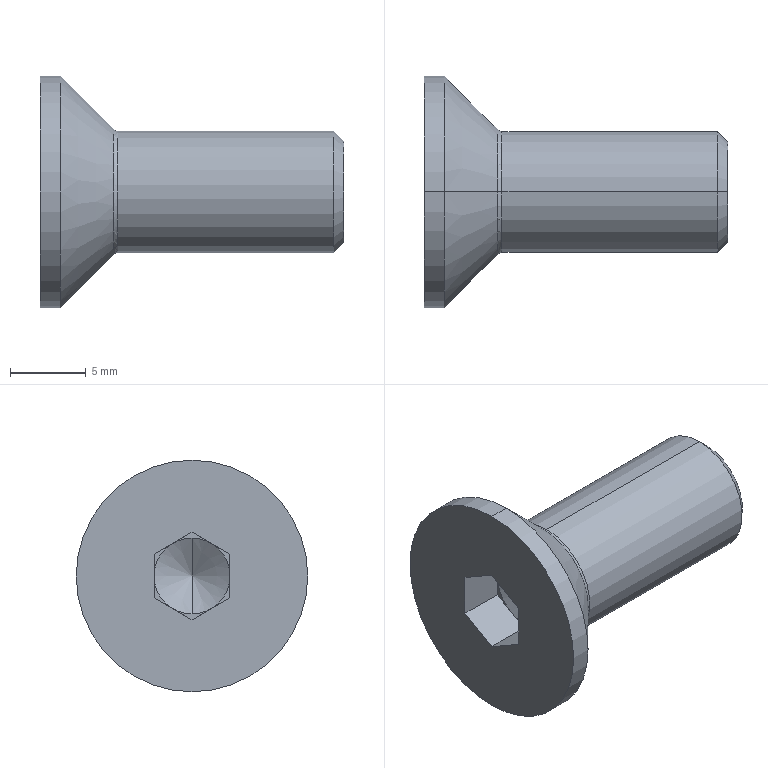Part | SolidWorks | features RevCut 3, Chamfer 1, Cut 1, Fillet 1, LPattern 1, Revolution 1 | 1 solid | 26 faces | box 20 x 15.24 x 15.24 mm | volume 1317 mm3 | plane 14 | cone 6 | cylinder 4 | torus 2 | commonest cylinder face diameters 8 x2 15.24 x2
STEP:
#1=CARTESIAN_POINT('',(4.443,0.,0.));
#2=VERTEX_POINT('',#1);
#3=CARTESIAN_POINT('',(3.,0.,2.5));
#4=VERTEX_POINT('',#3);
#5=CARTESIAN_POINT('',(4.443,0.,0.));
#6=DIRECTION('',(-0.5,0.,0.866));
#7=VECTOR('',#6,1000.);
#8=LINE('',#5,#7);
#9=EDGE_CURVE('',#2,#4,#8,.T.);
#10=ORIENTED_EDGE('',*,*,#9,.F.);
#11=CARTESIAN_POINT('',(3.,0.,-2.5));
#12=VERTEX_POINT('',#11);
#13=CARTESIAN_POINT('',(4.443,0.,0.));
#14=DIRECTION('',(-0.5,0.,-0.866));
#15=VECTOR('',#14,1000.);
#16=LINE('',#13,#15);
#17=EDGE_CURVE('',#2,#12,#16,.T.);
#18=ORIENTED_EDGE('',*,*,#17,.T.);
#19=CARTESIAN_POINT('',(3.,-1.25,-2.165));
#20=VERTEX_POINT('',#19);
#21=CARTESIAN_POINT('',(3.,0.,0.));
#22=DIRECTION('',(-1.,0.,0.));
#23=DIRECTION('',(0.,0.,1.));
#24=AXIS2_PLACEMENT_3D('',#21,#22,#23);
#25=CIRCLE('',#24,2.5);
#26=EDGE_CURVE('',#12,#20,#25,.T.);
#27=ORIENTED_EDGE('',*,*,#26,.T.);
#28=CARTESIAN_POINT('',(3.,-2.5,0.));
#29=VERTEX_POINT('',#28);
#30=CARTESIAN_POINT('',(3.,0.,0.));
#31=DIRECTION('',(-1.,0.,0.));
#32=DIRECTION('',(0.,0.,1.));
#33=AXIS2_PLACEMENT_3D('',#30,#31,#32);
#34=CIRCLE('',#33,2.5);
#35=EDGE_CURVE('',#20,#29,#34,.T.);
#36=ORIENTED_EDGE('',*,*,#35,.T.);
#37=CARTESIAN_POINT('',(3.,-1.25,2.165));
#38=VERTEX_POINT('',#37);
#39=CARTESIAN_POINT('',(3.,0.,0.));
#40=DIRECTION('',(-1.,0.,0.));
#41=DIRECTION('',(0.,0.,1.));
#42=AXIS2_PLACEMENT_3D('',#39,#40,#41);
#43=CIRCLE('',#42,2.5);
#44=EDGE_CURVE('',#29,#38,#43,.T.);
#45=ORIENTED_EDGE('',*,*,#44,.T.);
#46=CARTESIAN_POINT('',(3.,0.,0.));
#47=DIRECTION('',(-1.,0.,0.));
#48=DIRECTION('',(0.,0.,1.));
#49=AXIS2_PLACEMENT_3D('',#46,#47,#48);
#50=CIRCLE('',#49,2.5);
#51=EDGE_CURVE('',#38,#4,#50,.T.);
#52=ORIENTED_EDGE('',*,*,#51,.T.);
#53=EDGE_LOOP('',(#10,#18,#27,#36,#45,#52));
#54=FACE_OUTER_BOUND('',#53,.T.);
#55=CARTESIAN_POINT('',(-995.557,0.,0.));
#56=DIRECTION('',(-1.,0.,0.));
#57=DIRECTION('',(0.,0.,1.));
#58=AXIS2_PLACEMENT_3D('',#55,#56,#57);
#59=CONICAL_SURFACE('',#58,1732.051,1.047);
#60=ADVANCED_FACE('',(#54),#59,.F.);
#61=CARTESIAN_POINT('',(0.,0.,7.62));
#62=VERTEX_POINT('',#61);
#63=CARTESIAN_POINT('',(0.,0.,-7.62));
#64=VERTEX_POINT('',#63);
#65=CARTESIAN_POINT('',(0.,0.,0.));
#66=DIRECTION('',(-1.,0.,0.));
#67=DIRECTION('',(0.,0.,-1.));
#68=AXIS2_PLACEMENT_3D('',#65,#66,#67);
#69=CIRCLE('',#68,7.62);
#70=EDGE_CURVE('',#62,#64,#69,.T.);
#71=ORIENTED_EDGE('',*,*,#70,.F.);
#72=CARTESIAN_POINT('',(1.34,0.,7.62));
#73=VERTEX_POINT('',#72);
#74=CARTESIAN_POINT('',(11.853,0.,7.62));
#75=DIRECTION('',(1.,0.,0.));
#76=VECTOR('',#75,1000.);
#77=LINE('',#74,#76);
#78=EDGE_CURVE('',#62,#73,#77,.T.);
#79=ORIENTED_EDGE('',*,*,#78,.T.);
#80=CARTESIAN_POINT('',(1.34,0.,-7.62));
#81=VERTEX_POINT('',#80);
#82=CARTESIAN_POINT('',(1.34,0.,0.));
#83=DIRECTION('',(1.,0.,0.));
#84=DIRECTION('',(0.,0.,1.));
#85=AXIS2_PLACEMENT_3D('',#82,#83,#84);
#86=CIRCLE('',#85,7.62);
#87=EDGE_CURVE('',#81,#73,#86,.T.);
#88=ORIENTED_EDGE('',*,*,#87,.F.);
#89=CARTESIAN_POINT('',(11.853,0.,-7.62));
#90=DIRECTION('',(1.,0.,0.));
#91=VECTOR('',#90,1000.);
#92=LINE('',#89,#91);
#93=EDGE_CURVE('',#64,#81,#92,.T.);
#94=ORIENTED_EDGE('',*,*,#93,.F.);
#95=EDGE_LOOP('',(#71,#79,#88,#94));
#96=FACE_OUTER_BOUND('',#95,.T.);
#97=CARTESIAN_POINT('',(11.853,0.,0.));
#98=DIRECTION('',(1.,0.,0.));
#99=DIRECTION('',(0.,0.,-1.));
#100=AXIS2_PLACEMENT_3D('',#97,#98,#99);
#101=CYLINDRICAL_SURFACE('',#100,7.62);
#102=ADVANCED_FACE('',(#96),#101,.T.);
#103=CARTESIAN_POINT('',(20.,0.,-3.323));
#104=VERTEX_POINT('',#103);
#105=CARTESIAN_POINT('',(20.,0.,3.323));
#106=VERTEX_POINT('',#105);
#107=CARTESIAN_POINT('',(20.,0.,0.));
#108=DIRECTION('',(1.,0.,0.));
#109=DIRECTION('',(0.,0.,1.));
#110=AXIS2_PLACEMENT_3D('',#107,#108,#109);
#111=CIRCLE('',#110,3.323);
#112=EDGE_CURVE('',#104,#106,#111,.T.);
#113=ORIENTED_EDGE('',*,*,#112,.F.);
#114=CARTESIAN_POINT('',(19.323,0.,-4.));
#115=VERTEX_POINT('',#114);
#116=CARTESIAN_POINT('',(19.323,0.,-4.));
#117=DIRECTION('',(-0.7071,0.,-0.7071));
#118=VECTOR('',#117,1000.);
#119=LINE('',#116,#118);
#120=EDGE_CURVE('',#104,#115,#119,.T.);
#121=ORIENTED_EDGE('',*,*,#120,.T.);
#122=CARTESIAN_POINT('',(19.323,0.,4.));
#123=VERTEX_POINT('',#122);
#124=CARTESIAN_POINT('',(19.323,0.,0.));
#125=DIRECTION('',(-1.,0.,0.));
#126=DIRECTION('',(0.,0.,1.));
#127=AXIS2_PLACEMENT_3D('',#124,#125,#126);
#128=CIRCLE('',#127,4.);
#129=EDGE_CURVE('',#123,#115,#128,.T.);
#130=ORIENTED_EDGE('',*,*,#129,.F.);
#131=CARTESIAN_POINT('',(19.323,0.,4.));
#132=DIRECTION('',(-0.7071,0.,0.7071));
#133=VECTOR('',#132,1000.);
#134=LINE('',#131,#133);
#135=EDGE_CURVE('',#106,#123,#134,.T.);
#136=ORIENTED_EDGE('',*,*,#135,.F.);
#137=EDGE_LOOP('',(#113,#121,#130,#136));
#138=FACE_OUTER_BOUND('',#137,.T.);
#139=CARTESIAN_POINT('',(19.323,0.,0.));
#140=DIRECTION('',(-1.,0.,0.));
#141=DIRECTION('',(0.,0.,1.));
#142=AXIS2_PLACEMENT_3D('',#139,#140,#141);
#143=CONICAL_SURFACE('',#142,4.,0.7854);
#144=ADVANCED_FACE('',(#138),#143,.T.);
#145=CARTESIAN_POINT('',(4.843,0.,-4.117));
#146=VERTEX_POINT('',#145);
#147=CARTESIAN_POINT('',(4.843,0.,4.117));
#148=VERTEX_POINT('',#147);
#149=CARTESIAN_POINT('',(4.843,0.,0.));
#150=DIRECTION('',(-1.,0.,0.));
#151=DIRECTION('',(0.,0.,1.));
#152=AXIS2_PLACEMENT_3D('',#149,#150,#151);
#153=CIRCLE('',#152,4.117);
#154=EDGE_CURVE('',#146,#148,#153,.T.);
#155=ORIENTED_EDGE('',*,*,#154,.F.);
#156=CARTESIAN_POINT('',(5.126,0.,-4.));
#157=VERTEX_POINT('',#156);
#158=CARTESIAN_POINT('',(5.126,0.,-4.4));
#159=DIRECTION('',(0.,1.,0.));
#160=DIRECTION('',(0.,0.,1.));
#161=AXIS2_PLACEMENT_3D('',#158,#159,#160);
#162=CIRCLE('',#161,0.4);
#163=EDGE_CURVE('',#146,#157,#162,.T.);
#164=ORIENTED_EDGE('',*,*,#163,.T.);
#165=CARTESIAN_POINT('',(5.126,0.,4.));
#166=VERTEX_POINT('',#165);
#167=CARTESIAN_POINT('',(5.126,0.,0.));
#168=DIRECTION('',(1.,0.,0.));
#169=DIRECTION('',(0.,0.,1.));
#170=AXIS2_PLACEMENT_3D('',#167,#168,#169);
#171=CIRCLE('',#170,4.);
#172=EDGE_CURVE('',#166,#157,#171,.T.);
#173=ORIENTED_EDGE('',*,*,#172,.F.);
#174=CARTESIAN_POINT('',(5.126,0.,4.4));
#175=DIRECTION('',(0.,-1.,0.));
#176=DIRECTION('',(0.,0.,-1.));
#177=AXIS2_PLACEMENT_3D('',#174,#175,#176);
#178=CIRCLE('',#177,0.4);
#179=EDGE_CURVE('',#148,#166,#178,.T.);
#180=ORIENTED_EDGE('',*,*,#179,.F.);
#181=EDGE_LOOP('',(#155,#164,#173,#180));
#182=FACE_OUTER_BOUND('',#181,.T.);
#183=CARTESIAN_POINT('',(5.126,0.,0.));
#184=DIRECTION('',(-1.,0.,0.));
#185=DIRECTION('',(0.,0.,1.));
#186=AXIS2_PLACEMENT_3D('',#183,#184,#185);
#187=TOROIDAL_SURFACE('',#186,4.4,0.4);
#188=ADVANCED_FACE('',(#182),#187,.F.);
#189=ORIENTED_EDGE('',*,*,#129,.T.);
#190=CARTESIAN_POINT('',(-0.5871,0.,-4.));
#191=DIRECTION('',(-1.,0.,0.));
#192=VECTOR('',#191,1000.);
#193=LINE('',#190,#192);
#194=EDGE_CURVE('',#115,#157,#193,.T.);
#195=ORIENTED_EDGE('',*,*,#194,.T.);
#196=CARTESIAN_POINT('',(5.126,0.,0.));
#197=DIRECTION('',(1.,0.,0.));
#198=DIRECTION('',(0.,0.,1.));
#199=AXIS2_PLACEMENT_3D('',#196,#197,#198);
#200=CIRCLE('',#199,4.);
#201=EDGE_CURVE('',#157,#166,#200,.T.);
#202=ORIENTED_EDGE('',*,*,#201,.T.);
#203=CARTESIAN_POINT('',(-0.5871,0.,4.));
#204=DIRECTION('',(-1.,0.,0.));
#205=VECTOR('',#204,1000.);
#206=LINE('',#203,#205);
#207=EDGE_CURVE('',#123,#166,#206,.T.);
#208=ORIENTED_EDGE('',*,*,#207,.F.);
#209=EDGE_LOOP('',(#189,#195,#202,#208));
#210=FACE_OUTER_BOUND('',#209,.T.);
#211=CARTESIAN_POINT('',(-0.5871,0.,0.));
#212=DIRECTION('',(-1.,0.,0.));
#213=DIRECTION('',(0.,0.,1.));
#214=AXIS2_PLACEMENT_3D('',#211,#212,#213);
#215=CYLINDRICAL_SURFACE('',#214,4.);
#216=ADVANCED_FACE('',(#210),#215,.T.);
#217=CARTESIAN_POINT('',(4.843,0.,0.));
#218=DIRECTION('',(-1.,0.,0.));
#219=DIRECTION('',(0.,0.,1.));
#220=AXIS2_PLACEMENT_3D('',#217,#218,#219);
#221=CIRCLE('',#220,4.117);
#222=EDGE_CURVE('',#148,#146,#221,.T.);
#223=ORIENTED_EDGE('',*,*,#222,.T.);
#224=CARTESIAN_POINT('',(4.96,0.,-4.));
#225=DIRECTION('',(-0.7071,0.,-0.7071));
#226=VECTOR('',#225,1000.);
#227=LINE('',#224,#226);
#228=EDGE_CURVE('',#146,#81,#227,.T.);
#229=ORIENTED_EDGE('',*,*,#228,.T.);
#230=ORIENTED_EDGE('',*,*,#87,.T.);
#231=CARTESIAN_POINT('',(4.96,0.,4.));
#232=DIRECTION('',(-0.7071,0.,0.7071));
#233=VECTOR('',#232,1000.);
#234=LINE('',#231,#233);
#235=EDGE_CURVE('',#148,#73,#234,.T.);
#236=ORIENTED_EDGE('',*,*,#235,.F.);
#237=EDGE_LOOP('',(#223,#229,#230,#236));
#238=FACE_OUTER_BOUND('',#237,.T.);
#239=CARTESIAN_POINT('',(4.96,0.,0.));
#240=DIRECTION('',(-1.,0.,0.));
#241=DIRECTION('',(0.,0.,1.));
#242=AXIS2_PLACEMENT_3D('',#239,#240,#241);
#243=CONICAL_SURFACE('',#242,4.,0.7854);
#244=ADVANCED_FACE('',(#238),#243,.T.);
#245=ORIENTED_EDGE('',*,*,#228,.F.);
#246=ORIENTED_EDGE('',*,*,#154,.T.);
#247=ORIENTED_EDGE('',*,*,#235,.T.);
#248=CARTESIAN_POINT('',(1.34,0.,0.));
#249=DIRECTION('',(1.,0.,0.));
#250=DIRECTION('',(0.,0.,1.));
#251=AXIS2_PLACEMENT_3D('',#248,#249,#250);
#252=CIRCLE('',#251,7.62);
#253=EDGE_CURVE('',#73,#81,#252,.T.);
#254=ORIENTED_EDGE('',*,*,#253,.T.);
#255=EDGE_LOOP('',(#245,#246,#247,#254));
#256=FACE_OUTER_BOUND('',#255,.T.);
#257=CARTESIAN_POINT('',(4.96,0.,0.));
#258=DIRECTION('',(-1.,0.,0.));
#259=DIRECTION('',(0.,0.,1.));
#260=AXIS2_PLACEMENT_3D('',#257,#258,#259);
#261=CONICAL_SURFACE('',#260,4.,0.7854);
#262=ADVANCED_FACE('',(#256),#261,.T.);
#263=ORIENTED_EDGE('',*,*,#194,.F.);
#264=CARTESIAN_POINT('',(19.323,0.,0.));
#265=DIRECTION('',(-1.,0.,0.));
#266=DIRECTION('',(0.,0.,1.));
#267=AXIS2_PLACEMENT_3D('',#264,#265,#266);
#268=CIRCLE('',#267,4.);
#269=EDGE_CURVE('',#115,#123,#268,.T.);
#270=ORIENTED_EDGE('',*,*,#269,.T.);
#271=ORIENTED_EDGE('',*,*,#207,.T.);
#272=ORIENTED_EDGE('',*,*,#172,.T.);
#273=EDGE_LOOP('',(#263,#270,#271,#272));
#274=FACE_OUTER_BOUND('',#273,.T.);
#275=CARTESIAN_POINT('',(-0.5871,0.,0.));
#276=DIRECTION('',(-1.,0.,0.));
#277=DIRECTION('',(0.,0.,1.));
#278=AXIS2_PLACEMENT_3D('',#275,#276,#277);
#279=CYLINDRICAL_SURFACE('',#278,4.);
#280=ADVANCED_FACE('',(#274),#279,.T.);
#281=CARTESIAN_POINT('',(20.,0.,0.));
#282=DIRECTION('',(1.,0.,0.));
#283=DIRECTION('',(0.,0.,1.));
#284=AXIS2_PLACEMENT_3D('',#281,#282,#283);
#285=CIRCLE('',#284,3.323);
#286=EDGE_CURVE('',#106,#104,#285,.T.);
#287=ORIENTED_EDGE('',*,*,#286,.T.);
#288=ORIENTED_EDGE('',*,*,#112,.T.);
#289=EDGE_LOOP('',(#287,#288));
#290=FACE_OUTER_BOUND('',#289,.T.);
#291=CARTESIAN_POINT('',(20.,4.,0.));
#292=DIRECTION('',(-1.,0.,0.));
#293=DIRECTION('',(0.,0.,1.));
#294=AXIS2_PLACEMENT_3D('',#291,#292,#293);
#295=PLANE('',#294);
#296=ADVANCED_FACE('',(#290),#295,.F.);
#297=ORIENTED_EDGE('',*,*,#163,.F.);
#298=ORIENTED_EDGE('',*,*,#222,.F.);
#299=ORIENTED_EDGE('',*,*,#179,.T.);
#300=ORIENTED_EDGE('',*,*,#201,.F.);
#301=EDGE_LOOP('',(#297,#298,#299,#300));
#302=FACE_OUTER_BOUND('',#301,.T.);
#303=CARTESIAN_POINT('',(5.126,0.,0.));
#304=DIRECTION('',(-1.,0.,0.));
#305=DIRECTION('',(0.,0.,1.));
#306=AXIS2_PLACEMENT_3D('',#303,#304,#305);
#307=TOROIDAL_SURFACE('',#306,4.4,0.4);
#308=ADVANCED_FACE('',(#302),#307,.F.);
#309=ORIENTED_EDGE('',*,*,#120,.F.);
#310=ORIENTED_EDGE('',*,*,#286,.F.);
#311=ORIENTED_EDGE('',*,*,#135,.T.);
#312=ORIENTED_EDGE('',*,*,#269,.F.);
#313=EDGE_LOOP('',(#309,#310,#311,#312));
#314=FACE_OUTER_BOUND('',#313,.T.);
#315=CARTESIAN_POINT('',(19.323,0.,0.));
#316=DIRECTION('',(-1.,0.,0.));
#317=DIRECTION('',(0.,0.,1.));
#318=AXIS2_PLACEMENT_3D('',#315,#316,#317);
#319=CONICAL_SURFACE('',#318,4.,0.7854);
#320=ADVANCED_FACE('',(#314),#319,.T.);
#321=ORIENTED_EDGE('',*,*,#78,.F.);
#322=CARTESIAN_POINT('',(0.,0.,0.));
#323=DIRECTION('',(-1.,0.,0.));
#324=DIRECTION('',(0.,0.,-1.));
#325=AXIS2_PLACEMENT_3D('',#322,#323,#324);
#326=CIRCLE('',#325,7.62);
#327=EDGE_CURVE('',#64,#62,#326,.T.);
#328=ORIENTED_EDGE('',*,*,#327,.F.);
#329=ORIENTED_EDGE('',*,*,#93,.T.);
#330=ORIENTED_EDGE('',*,*,#253,.F.);
#331=EDGE_LOOP('',(#321,#328,#329,#330));
#332=FACE_OUTER_BOUND('',#331,.T.);
#333=CARTESIAN_POINT('',(11.853,0.,0.));
#334=DIRECTION('',(1.,0.,0.));
#335=DIRECTION('',(0.,0.,-1.));
#336=AXIS2_PLACEMENT_3D('',#333,#334,#335);
#337=CYLINDRICAL_SURFACE('',#336,7.62);
#338=ADVANCED_FACE('',(#332),#337,.T.);
#339=ORIENTED_EDGE('',*,*,#17,.F.);
#340=ORIENTED_EDGE('',*,*,#9,.T.);
#341=CARTESIAN_POINT('',(3.,1.25,2.165));
#342=VERTEX_POINT('',#341);
#343=CARTESIAN_POINT('',(3.,0.,0.));
#344=DIRECTION('',(-1.,0.,0.));
#345=DIRECTION('',(0.,0.,1.));
#346=AXIS2_PLACEMENT_3D('',#343,#344,#345);
#347=CIRCLE('',#346,2.5);
#348=EDGE_CURVE('',#4,#342,#347,.T.);
#349=ORIENTED_EDGE('',*,*,#348,.T.);
#350=CARTESIAN_POINT('',(3.,2.5,0.));
#351=VERTEX_POINT('',#350);
#352=CARTESIAN_POINT('',(3.,0.,0.));
#353=DIRECTION('',(-1.,0.,0.));
#354=DIRECTION('',(0.,0.,1.));
#355=AXIS2_PLACEMENT_3D('',#352,#353,#354);
#356=CIRCLE('',#355,2.5);
#357=EDGE_CURVE('',#342,#351,#356,.T.);
#358=ORIENTED_EDGE('',*,*,#357,.T.);
#359=CARTESIAN_POINT('',(3.,1.25,-2.165));
#360=VERTEX_POINT('',#359);
#361=CARTESIAN_POINT('',(3.,0.,0.));
#362=DIRECTION('',(-1.,0.,0.));
#363=DIRECTION('',(0.,0.,1.));
#364=AXIS2_PLACEMENT_3D('',#361,#362,#363);
#365=CIRCLE('',#364,2.5);
#366=EDGE_CURVE('',#351,#360,#365,.T.);
#367=ORIENTED_EDGE('',*,*,#366,.T.);
#368=CARTESIAN_POINT('',(3.,0.,0.));
#369=DIRECTION('',(-1.,0.,0.));
#370=DIRECTION('',(0.,0.,1.));
#371=AXIS2_PLACEMENT_3D('',#368,#369,#370);
#372=CIRCLE('',#371,2.5);
#373=EDGE_CURVE('',#360,#12,#372,.T.);
#374=ORIENTED_EDGE('',*,*,#373,.T.);
#375=EDGE_LOOP('',(#339,#340,#349,#358,#367,#374));
#376=FACE_OUTER_BOUND('',#375,.T.);
#377=CARTESIAN_POINT('',(-995.557,0.,0.));
#378=DIRECTION('',(-1.,0.,0.));
#379=DIRECTION('',(0.,0.,1.));
#380=AXIS2_PLACEMENT_3D('',#377,#378,#379);
#381=CONICAL_SURFACE('',#380,1732.051,1.047);
#382=ADVANCED_FACE('',(#376),#381,.F.);
#383=ORIENTED_EDGE('',*,*,#44,.F.);
#384=CARTESIAN_POINT('',(3.,-2.5,1.443));
#385=VERTEX_POINT('',#384);
#386=CARTESIAN_POINT('',(3.,-2.5,1.443));
#387=DIRECTION('',(0.,0.,-1.));
#388=VECTOR('',#387,1000.);
#389=LINE('',#386,#388);
#390=EDGE_CURVE('',#385,#29,#389,.T.);
#391=ORIENTED_EDGE('',*,*,#390,.F.);
#392=CARTESIAN_POINT('',(3.,0.,2.887));
#393=DIRECTION('',(0.,-0.866,-0.5));
#394=VECTOR('',#393,1000.);
#395=LINE('',#392,#394);
#396=EDGE_CURVE('',#38,#385,#395,.T.);
#397=ORIENTED_EDGE('',*,*,#396,.F.);
#398=EDGE_LOOP('',(#383,#391,#397));
#399=FACE_OUTER_BOUND('',#398,.T.);
#400=CARTESIAN_POINT('',(3.,0.,-2.887));
#401=DIRECTION('',(1.,0.,0.));
#402=DIRECTION('',(0.,0.,-1.));
#403=AXIS2_PLACEMENT_3D('',#400,#401,#402);
#404=PLANE('',#403);
#405=ADVANCED_FACE('',(#399),#404,.F.);
#406=ORIENTED_EDGE('',*,*,#51,.F.);
#407=CARTESIAN_POINT('',(3.,0.,2.887));
#408=VERTEX_POINT('',#407);
#409=CARTESIAN_POINT('',(3.,0.,2.887));
#410=DIRECTION('',(0.,-0.866,-0.5));
#411=VECTOR('',#410,1000.);
#412=LINE('',#409,#411);
#413=EDGE_CURVE('',#408,#38,#412,.T.);
#414=ORIENTED_EDGE('',*,*,#413,.F.);
#415=CARTESIAN_POINT('',(3.,2.5,1.443));
#416=DIRECTION('',(0.,-0.866,0.5));
#417=VECTOR('',#416,1000.);
#418=LINE('',#415,#417);
#419=EDGE_CURVE('',#342,#408,#418,.T.);
#420=ORIENTED_EDGE('',*,*,#419,.F.);
#421=ORIENTED_EDGE('',*,*,#348,.F.);
#422=EDGE_LOOP('',(#406,#414,#420,#421));
#423=FACE_OUTER_BOUND('',#422,.T.);
#424=CARTESIAN_POINT('',(3.,0.,-2.887));
#425=DIRECTION('',(1.,0.,0.));
#426=DIRECTION('',(0.,0.,-1.));
#427=AXIS2_PLACEMENT_3D('',#424,#425,#426);
#428=PLANE('',#427);
#429=ADVANCED_FACE('',(#423),#428,.F.);
#430=ORIENTED_EDGE('',*,*,#357,.F.);
#431=CARTESIAN_POINT('',(3.,2.5,1.443));
#432=VERTEX_POINT('',#431);
#433=CARTESIAN_POINT('',(3.,2.5,1.443));
#434=DIRECTION('',(0.,-0.866,0.5));
#435=VECTOR('',#434,1000.);
#436=LINE('',#433,#435);
#437=EDGE_CURVE('',#432,#342,#436,.T.);
#438=ORIENTED_EDGE('',*,*,#437,.F.);
#439=CARTESIAN_POINT('',(3.,2.5,-1.443));
#440=DIRECTION('',(0.,0.,1.));
#441=VECTOR('',#440,1000.);
#442=LINE('',#439,#441);
#443=EDGE_CURVE('',#351,#432,#442,.T.);
#444=ORIENTED_EDGE('',*,*,#443,.F.);
#445=EDGE_LOOP('',(#430,#438,#444));
#446=FACE_OUTER_BOUND('',#445,.T.);
#447=CARTESIAN_POINT('',(3.,0.,-2.887));
#448=DIRECTION('',(1.,0.,0.));
#449=DIRECTION('',(0.,0.,-1.));
#450=AXIS2_PLACEMENT_3D('',#447,#448,#449);
#451=PLANE('',#450);
#452=ADVANCED_FACE('',(#446),#451,.F.);
#453=ORIENTED_EDGE('',*,*,#366,.F.);
#454=CARTESIAN_POINT('',(3.,2.5,-1.443));
#455=VERTEX_POINT('',#454);
#456=CARTESIAN_POINT('',(3.,2.5,-1.443));
#457=DIRECTION('',(0.,0.,1.));
#458=VECTOR('',#457,1000.);
#459=LINE('',#456,#458);
#460=EDGE_CURVE('',#455,#351,#459,.T.);
#461=ORIENTED_EDGE('',*,*,#460,.F.);
#462=CARTESIAN_POINT('',(3.,0.,-2.887));
#463=DIRECTION('',(0.,0.866,0.5));
#464=VECTOR('',#463,1000.);
#465=LINE('',#462,#464);
#466=EDGE_CURVE('',#360,#455,#465,.T.);
#467=ORIENTED_EDGE('',*,*,#466,.F.);
#468=EDGE_LOOP('',(#453,#461,#467));
#469=FACE_OUTER_BOUND('',#468,.T.);
#470=CARTESIAN_POINT('',(3.,0.,-2.887));
#471=DIRECTION('',(1.,0.,0.));
#472=DIRECTION('',(0.,0.,-1.));
#473=AXIS2_PLACEMENT_3D('',#470,#471,#472);
#474=PLANE('',#473);
#475=ADVANCED_FACE('',(#469),#474,.F.);
#476=ORIENTED_EDGE('',*,*,#373,.F.);
#477=CARTESIAN_POINT('',(3.,0.,-2.887));
#478=VERTEX_POINT('',#477);
#479=CARTESIAN_POINT('',(3.,0.,-2.887));
#480=DIRECTION('',(0.,0.866,0.5));
#481=VECTOR('',#480,1000.);
#482=LINE('',#479,#481);
#483=EDGE_CURVE('',#478,#360,#482,.T.);
#484=ORIENTED_EDGE('',*,*,#483,.F.);
#485=CARTESIAN_POINT('',(3.,-2.5,-1.443));
#486=DIRECTION('',(0.,0.866,-0.5));
#487=VECTOR('',#486,1000.);
#488=LINE('',#485,#487);
#489=EDGE_CURVE('',#20,#478,#488,.T.);
#490=ORIENTED_EDGE('',*,*,#489,.F.);
#491=ORIENTED_EDGE('',*,*,#26,.F.);
#492=EDGE_LOOP('',(#476,#484,#490,#491));
#493=FACE_OUTER_BOUND('',#492,.T.);
#494=CARTESIAN_POINT('',(3.,0.,-2.887));
#495=DIRECTION('',(1.,0.,0.));
#496=DIRECTION('',(0.,0.,-1.));
#497=AXIS2_PLACEMENT_3D('',#494,#495,#496);
#498=PLANE('',#497);
#499=ADVANCED_FACE('',(#493),#498,.F.);
#500=ORIENTED_EDGE('',*,*,#35,.F.);
#501=CARTESIAN_POINT('',(3.,-2.5,-1.443));
#502=VERTEX_POINT('',#501);
#503=CARTESIAN_POINT('',(3.,-2.5,-1.443));
#504=DIRECTION('',(0.,0.866,-0.5));
#505=VECTOR('',#504,1000.);
#506=LINE('',#503,#505);
#507=EDGE_CURVE('',#502,#20,#506,.T.);
#508=ORIENTED_EDGE('',*,*,#507,.F.);
#509=CARTESIAN_POINT('',(3.,-2.5,1.443));
#510=DIRECTION('',(0.,0.,-1.));
#511=VECTOR('',#510,1000.);
#512=LINE('',#509,#511);
#513=EDGE_CURVE('',#29,#502,#512,.T.);
#514=ORIENTED_EDGE('',*,*,#513,.F.);
#515=EDGE_LOOP('',(#500,#508,#514));
#516=FACE_OUTER_BOUND('',#515,.T.);
#517=CARTESIAN_POINT('',(3.,0.,-2.887));
#518=DIRECTION('',(1.,0.,0.));
#519=DIRECTION('',(0.,0.,-1.));
#520=AXIS2_PLACEMENT_3D('',#517,#518,#519);
#521=PLANE('',#520);
#522=ADVANCED_FACE('',(#516),#521,.F.);
#523=CARTESIAN_POINT('',(0.,-2.5,1.443));
#524=VERTEX_POINT('',#523);
#525=CARTESIAN_POINT('',(0.,-2.5,-1.443));
#526=VERTEX_POINT('',#525);
#527=CARTESIAN_POINT('',(0.,-2.5,1.443));
#528=DIRECTION('',(0.,0.,-1.));
#529=VECTOR('',#528,1000.);
#530=LINE('',#527,#529);
#531=EDGE_CURVE('',#524,#526,#530,.T.);
#532=ORIENTED_EDGE('',*,*,#531,.F.);
#533=CARTESIAN_POINT('',(3.,-2.5,1.443));
#534=DIRECTION('',(-1.,0.,0.));
#535=VECTOR('',#534,1000.);
#536=LINE('',#533,#535);
#537=EDGE_CURVE('',#385,#524,#536,.T.);
#538=ORIENTED_EDGE('',*,*,#537,.F.);
#539=ORIENTED_EDGE('',*,*,#390,.T.);
#540=ORIENTED_EDGE('',*,*,#513,.T.);
#541=CARTESIAN_POINT('',(3.,-2.5,-1.443));
#542=DIRECTION('',(-1.,0.,0.));
#543=VECTOR('',#542,1000.);
#544=LINE('',#541,#543);
#545=EDGE_CURVE('',#502,#526,#544,.T.);
#546=ORIENTED_EDGE('',*,*,#545,.T.);
#547=EDGE_LOOP('',(#532,#538,#539,#540,#546));
#548=FACE_OUTER_BOUND('',#547,.T.);
#549=CARTESIAN_POINT('',(3.,-2.5,1.443));
#550=DIRECTION('',(0.,1.,0.));
#551=DIRECTION('',(0.,0.,1.));
#552=AXIS2_PLACEMENT_3D('',#549,#550,#551);
#553=PLANE('',#552);
#554=ADVANCED_FACE('',(#548),#553,.T.);
#555=CARTESIAN_POINT('',(0.,0.,2.887));
#556=VERTEX_POINT('',#555);
#557=CARTESIAN_POINT('',(0.,0.,2.887));
#558=DIRECTION('',(0.,-0.866,-0.5));
#559=VECTOR('',#558,1000.);
#560=LINE('',#557,#559);
#561=EDGE_CURVE('',#556,#524,#560,.T.);
#562=ORIENTED_EDGE('',*,*,#561,.F.);
#563=CARTESIAN_POINT('',(3.,0.,2.887));
#564=DIRECTION('',(-1.,0.,0.));
#565=VECTOR('',#564,1000.);
#566=LINE('',#563,#565);
#567=EDGE_CURVE('',#408,#556,#566,.T.);
#568=ORIENTED_EDGE('',*,*,#567,.F.);
#569=ORIENTED_EDGE('',*,*,#413,.T.);
#570=ORIENTED_EDGE('',*,*,#396,.T.);
#571=ORIENTED_EDGE('',*,*,#537,.T.);
#572=EDGE_LOOP('',(#562,#568,#569,#570,#571));
#573=FACE_OUTER_BOUND('',#572,.T.);
#574=CARTESIAN_POINT('',(3.,0.,2.887));
#575=DIRECTION('',(0.,0.5,-0.866));
#576=DIRECTION('',(0.,0.866,0.5));
#577=AXIS2_PLACEMENT_3D('',#574,#575,#576);
#578=PLANE('',#577);
#579=ADVANCED_FACE('',(#573),#578,.T.);
#580=CARTESIAN_POINT('',(0.,2.5,1.443));
#581=VERTEX_POINT('',#580);
#582=CARTESIAN_POINT('',(0.,2.5,1.443));
#583=DIRECTION('',(0.,-0.866,0.5));
#584=VECTOR('',#583,1000.);
#585=LINE('',#582,#584);
#586=EDGE_CURVE('',#581,#556,#585,.T.);
#587=ORIENTED_EDGE('',*,*,#586,.F.);
#588=CARTESIAN_POINT('',(3.,2.5,1.443));
#589=DIRECTION('',(-1.,0.,0.));
#590=VECTOR('',#589,1000.);
#591=LINE('',#588,#590);
#592=EDGE_CURVE('',#432,#581,#591,.T.);
#593=ORIENTED_EDGE('',*,*,#592,.F.);
#594=ORIENTED_EDGE('',*,*,#437,.T.);
#595=ORIENTED_EDGE('',*,*,#419,.T.);
#596=ORIENTED_EDGE('',*,*,#567,.T.);
#597=EDGE_LOOP('',(#587,#593,#594,#595,#596));
#598=FACE_OUTER_BOUND('',#597,.T.);
#599=CARTESIAN_POINT('',(3.,2.5,1.443));
#600=DIRECTION('',(0.,-0.5,-0.866));
#601=DIRECTION('',(0.,0.866,-0.5));
#602=AXIS2_PLACEMENT_3D('',#599,#600,#601);
#603=PLANE('',#602);
#604=ADVANCED_FACE('',(#598),#603,.T.);
#605=CARTESIAN_POINT('',(0.,2.5,-1.443));
#606=VERTEX_POINT('',#605);
#607=CARTESIAN_POINT('',(0.,2.5,-1.443));
#608=DIRECTION('',(0.,0.,1.));
#609=VECTOR('',#608,1000.);
#610=LINE('',#607,#609);
#611=EDGE_CURVE('',#606,#581,#610,.T.);
#612=ORIENTED_EDGE('',*,*,#611,.F.);
#613=CARTESIAN_POINT('',(3.,2.5,-1.443));
#614=DIRECTION('',(-1.,0.,0.));
#615=VECTOR('',#614,1000.);
#616=LINE('',#613,#615);
#617=EDGE_CURVE('',#455,#606,#616,.T.);
#618=ORIENTED_EDGE('',*,*,#617,.F.);
#619=ORIENTED_EDGE('',*,*,#460,.T.);
#620=ORIENTED_EDGE('',*,*,#443,.T.);
#621=ORIENTED_EDGE('',*,*,#592,.T.);
#622=EDGE_LOOP('',(#612,#618,#619,#620,#621));
#623=FACE_OUTER_BOUND('',#622,.T.);
#624=CARTESIAN_POINT('',(3.,2.5,-1.443));
#625=DIRECTION('',(0.,-1.,0.));
#626=DIRECTION('',(0.,0.,-1.));
#627=AXIS2_PLACEMENT_3D('',#624,#625,#626);
#628=PLANE('',#627);
#629=ADVANCED_FACE('',(#623),#628,.T.);
#630=CARTESIAN_POINT('',(0.,0.,-2.887));
#631=VERTEX_POINT('',#630);
#632=CARTESIAN_POINT('',(0.,0.,-2.887));
#633=DIRECTION('',(0.,0.866,0.5));
#634=VECTOR('',#633,1000.);
#635=LINE('',#632,#634);
#636=EDGE_CURVE('',#631,#606,#635,.T.);
#637=ORIENTED_EDGE('',*,*,#636,.F.);
#638=CARTESIAN_POINT('',(3.,0.,-2.887));
#639=DIRECTION('',(-1.,0.,0.));
#640=VECTOR('',#639,1000.);
#641=LINE('',#638,#640);
#642=EDGE_CURVE('',#478,#631,#641,.T.);
#643=ORIENTED_EDGE('',*,*,#642,.F.);
#644=ORIENTED_EDGE('',*,*,#483,.T.);
#645=ORIENTED_EDGE('',*,*,#466,.T.);
#646=ORIENTED_EDGE('',*,*,#617,.T.);
#647=EDGE_LOOP('',(#637,#643,#644,#645,#646));
#648=FACE_OUTER_BOUND('',#647,.T.);
#649=CARTESIAN_POINT('',(3.,0.,-2.887));
#650=DIRECTION('',(0.,-0.5,0.866));
#651=DIRECTION('',(0.,-0.866,-0.5));
#652=AXIS2_PLACEMENT_3D('',#649,#650,#651);
#653=PLANE('',#652);
#654=ADVANCED_FACE('',(#648),#653,.T.);
#655=CARTESIAN_POINT('',(0.,-2.5,-1.443));
#656=DIRECTION('',(0.,0.866,-0.5));
#657=VECTOR('',#656,1000.);
#658=LINE('',#655,#657);
#659=EDGE_CURVE('',#526,#631,#658,.T.);
#660=ORIENTED_EDGE('',*,*,#659,.F.);
#661=ORIENTED_EDGE('',*,*,#545,.F.);
#662=ORIENTED_EDGE('',*,*,#507,.T.);
#663=ORIENTED_EDGE('',*,*,#489,.T.);
#664=ORIENTED_EDGE('',*,*,#642,.T.);
#665=EDGE_LOOP('',(#660,#661,#662,#663,#664));
#666=FACE_OUTER_BOUND('',#665,.T.);
#667=CARTESIAN_POINT('',(3.,-2.5,-1.443));
#668=DIRECTION('',(0.,0.5,0.866));
#669=DIRECTION('',(0.,-0.866,0.5));
#670=AXIS2_PLACEMENT_3D('',#667,#668,#669);
#671=PLANE('',#670);
#672=ADVANCED_FACE('',(#666),#671,.T.);
#673=ORIENTED_EDGE('',*,*,#327,.T.);
#674=ORIENTED_EDGE('',*,*,#70,.T.);
#675=EDGE_LOOP('',(#673,#674));
#676=FACE_OUTER_BOUND('',#675,.T.);
#677=ORIENTED_EDGE('',*,*,#659,.T.);
#678=ORIENTED_EDGE('',*,*,#636,.T.);
#679=ORIENTED_EDGE('',*,*,#611,.T.);
#680=ORIENTED_EDGE('',*,*,#586,.T.);
#681=ORIENTED_EDGE('',*,*,#561,.T.);
#682=ORIENTED_EDGE('',*,*,#531,.T.);
#683=EDGE_LOOP('',(#677,#678,#679,#680,#681,#682));
#684=FACE_BOUND('',#683,.T.);
#685=CARTESIAN_POINT('',(0.,0.,0.));
#686=DIRECTION('',(1.,0.,0.));
#687=DIRECTION('',(0.,0.,-1.));
#688=AXIS2_PLACEMENT_3D('',#685,#686,#687);
#689=PLANE('',#688);
#690=ADVANCED_FACE('',(#676,#684),#689,.F.);
#691=CLOSED_SHELL('',(#60,#102,#144,#188,#216,#244,#262,#280,#296,#308,#320,#338,#382,#405,#429,#452,#475,#499,#522,#554,#579,#604,#629,#654,#672,#690));
#692=MANIFOLD_SOLID_BREP('',#691);
#693=CARTESIAN_POINT('',(0.,0.,0.));
#694=DIRECTION('',(0.,0.,1.));
#695=DIRECTION('',(1.,0.,0.));
#696=AXIS2_PLACEMENT_3D('',#693,#694,#695);
#697=(LENGTH_UNIT()NAMED_UNIT(*)SI_UNIT(.MILLI.,.METRE.));
#698=UNCERTAINTY_MEASURE_WITH_UNIT(LENGTH_MEASURE(0.00001),#697,'','');
#699=(NAMED_UNIT(*)PLANE_ANGLE_UNIT()SI_UNIT($,.RADIAN.));
#700=(NAMED_UNIT(*)SI_UNIT($,.STERADIAN.)SOLID_ANGLE_UNIT());
#701=(GEOMETRIC_REPRESENTATION_CONTEXT(3)GLOBAL_UNCERTAINTY_ASSIGNED_CONTEXT((#698))GLOBAL_UNIT_ASSIGNED_CONTEXT((#697,#699,#700))REPRESENTATION_CONTEXT('',''));
#702=ADVANCED_BREP_SHAPE_REPRESENTATION('',(#692,#696),#701);